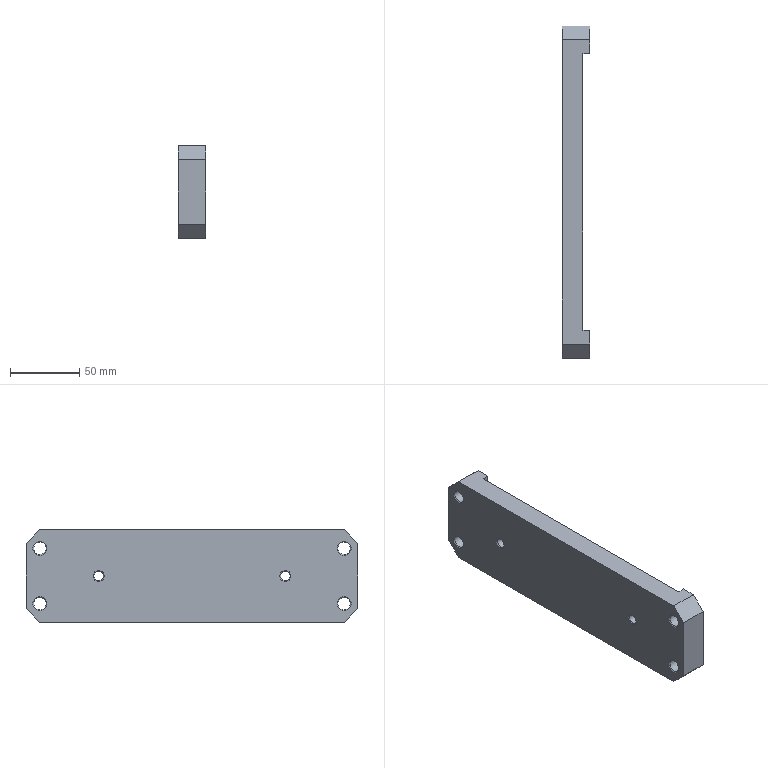Part | NX | features SIMPLE HOLE 6, DATUM_CSYS 5, SKETCH 4, EXTRUDE 2, HOLE PACKAGE 2, LINKED_CURVE 2, SYMBOLIC_THREAD 2, CHAMFER 1, LINKED_FACE 1 | 1 solid | 32 faces | box 20 x 240 x 67 mm | volume 244362 mm3 | plane 14 | cone 12 | cylinder 6 | commonest cylinder face diameters 9 x4 6.8 x2
STEP:
#1=CARTESIAN_POINT('',(85.,-110.,-450.));
#2=VERTEX_POINT('',#1);
#3=CARTESIAN_POINT('',(85.,-100.,-450.));
#4=VERTEX_POINT('',#3);
#5=CARTESIAN_POINT('',(85.,-120.,-450.));
#6=DIRECTION('',(0.,1.,0.));
#7=VECTOR('',#6,1000.);
#8=LINE('',#5,#7);
#9=EDGE_CURVE('',#2,#4,#8,.T.);
#10=ORIENTED_EDGE('',*,*,#9,.F.);
#11=CARTESIAN_POINT('',(65.,-110.,-450.));
#12=VERTEX_POINT('',#11);
#13=CARTESIAN_POINT('',(85.,-110.,-450.));
#14=DIRECTION('',(-1.,0.,0.));
#15=VECTOR('',#14,1000.);
#16=LINE('',#13,#15);
#17=EDGE_CURVE('',#2,#12,#16,.T.);
#18=ORIENTED_EDGE('',*,*,#17,.T.);
#19=CARTESIAN_POINT('',(65.,110.,-450.));
#20=VERTEX_POINT('',#19);
#21=CARTESIAN_POINT('',(65.,-120.,-450.));
#22=DIRECTION('',(0.,1.,0.));
#23=VECTOR('',#22,1000.);
#24=LINE('',#21,#23);
#25=EDGE_CURVE('',#12,#20,#24,.T.);
#26=ORIENTED_EDGE('',*,*,#25,.T.);
#27=CARTESIAN_POINT('',(85.,110.,-450.));
#28=VERTEX_POINT('',#27);
#29=CARTESIAN_POINT('',(85.,110.,-450.));
#30=DIRECTION('',(1.,0.,0.));
#31=VECTOR('',#30,1000.);
#32=LINE('',#29,#31);
#33=EDGE_CURVE('',#20,#28,#32,.T.);
#34=ORIENTED_EDGE('',*,*,#33,.T.);
#35=CARTESIAN_POINT('',(85.,100.,-450.));
#36=VERTEX_POINT('',#35);
#37=CARTESIAN_POINT('',(85.,-120.,-450.));
#38=DIRECTION('',(0.,1.,0.));
#39=VECTOR('',#38,1000.);
#40=LINE('',#37,#39);
#41=EDGE_CURVE('',#36,#28,#40,.T.);
#42=ORIENTED_EDGE('',*,*,#41,.F.);
#43=CARTESIAN_POINT('',(80.,100.,-450.));
#44=VERTEX_POINT('',#43);
#45=CARTESIAN_POINT('',(80.,100.,-450.));
#46=DIRECTION('',(1.,0.,0.));
#47=VECTOR('',#46,1000.);
#48=LINE('',#45,#47);
#49=EDGE_CURVE('',#44,#36,#48,.T.);
#50=ORIENTED_EDGE('',*,*,#49,.F.);
#51=CARTESIAN_POINT('',(80.,-100.,-450.));
#52=VERTEX_POINT('',#51);
#53=CARTESIAN_POINT('',(80.,-100.,-450.));
#54=DIRECTION('',(0.,1.,0.));
#55=VECTOR('',#54,1000.);
#56=LINE('',#53,#55);
#57=EDGE_CURVE('',#52,#44,#56,.T.);
#58=ORIENTED_EDGE('',*,*,#57,.F.);
#59=CARTESIAN_POINT('',(119.,-100.,-450.));
#60=DIRECTION('',(-1.,0.,0.));
#61=VECTOR('',#60,1000.);
#62=LINE('',#59,#61);
#63=EDGE_CURVE('',#4,#52,#62,.T.);
#64=ORIENTED_EDGE('',*,*,#63,.F.);
#65=EDGE_LOOP('',(#10,#18,#26,#34,#42,#50,#58,#64));
#66=FACE_BOUND('',#65,.T.);
#67=CARTESIAN_POINT('',(85.,-120.,-450.));
#68=DIRECTION('',(0.,0.,1.));
#69=DIRECTION('',(0.,-1.,0.));
#70=AXIS2_PLACEMENT_3D('',#67,#68,#69);
#71=PLANE('',#70);
#72=ADVANCED_FACE('',(#66),#71,.F.);
#73=CARTESIAN_POINT('',(85.,110.,-441.6));
#74=VERTEX_POINT('',#73);
#75=CARTESIAN_POINT('',(85.,110.,-436.5));
#76=DIRECTION('',(1.,0.,0.));
#77=DIRECTION('',(0.,0.,-1.));
#78=AXIS2_PLACEMENT_3D('',#75,#76,#77);
#79=CIRCLE('',#78,5.1);
#80=EDGE_CURVE('',#74,#74,#79,.F.);
#81=ORIENTED_EDGE('',*,*,#80,.T.);
#82=EDGE_LOOP('',(#81));
#83=FACE_BOUND('',#82,.T.);
#84=CARTESIAN_POINT('',(85.,110.,-401.6));
#85=VERTEX_POINT('',#84);
#86=CARTESIAN_POINT('',(85.,110.,-396.5));
#87=DIRECTION('',(1.,0.,0.));
#88=DIRECTION('',(0.,0.,-1.));
#89=AXIS2_PLACEMENT_3D('',#86,#87,#88);
#90=CIRCLE('',#89,5.1);
#91=EDGE_CURVE('',#85,#85,#90,.F.);
#92=ORIENTED_EDGE('',*,*,#91,.T.);
#93=EDGE_LOOP('',(#92));
#94=FACE_BOUND('',#93,.T.);
#95=CARTESIAN_POINT('',(85.,120.,-440.));
#96=VERTEX_POINT('',#95);
#97=CARTESIAN_POINT('',(85.,120.,-393.));
#98=VERTEX_POINT('',#97);
#99=CARTESIAN_POINT('',(85.,120.,-450.));
#100=DIRECTION('',(0.,0.,1.));
#101=VECTOR('',#100,1000.);
#102=LINE('',#99,#101);
#103=EDGE_CURVE('',#96,#98,#102,.T.);
#104=ORIENTED_EDGE('',*,*,#103,.T.);
#105=CARTESIAN_POINT('',(85.,110.,-383.));
#106=VERTEX_POINT('',#105);
#107=CARTESIAN_POINT('',(85.,-136.5,-136.5));
#108=DIRECTION('',(0.,0.7071,-0.7071));
#109=VECTOR('',#108,1000.);
#110=LINE('',#107,#109);
#111=EDGE_CURVE('',#98,#106,#110,.F.);
#112=ORIENTED_EDGE('',*,*,#111,.T.);
#113=CARTESIAN_POINT('',(85.,100.,-383.));
#114=VERTEX_POINT('',#113);
#115=CARTESIAN_POINT('',(85.,120.,-383.));
#116=DIRECTION('',(0.,-1.,0.));
#117=VECTOR('',#116,1000.);
#118=LINE('',#115,#117);
#119=EDGE_CURVE('',#106,#114,#118,.T.);
#120=ORIENTED_EDGE('',*,*,#119,.T.);
#121=CARTESIAN_POINT('',(85.,100.,0.));
#122=DIRECTION('',(0.,0.,1.));
#123=VECTOR('',#122,1000.);
#124=LINE('',#121,#123);
#125=EDGE_CURVE('',#36,#114,#124,.T.);
#126=ORIENTED_EDGE('',*,*,#125,.F.);
#127=ORIENTED_EDGE('',*,*,#41,.T.);
#128=CARTESIAN_POINT('',(85.,280.,-280.));
#129=DIRECTION('',(0.,-0.7071,-0.7071));
#130=VECTOR('',#129,1000.);
#131=LINE('',#128,#130);
#132=EDGE_CURVE('',#28,#96,#131,.F.);
#133=ORIENTED_EDGE('',*,*,#132,.T.);
#134=EDGE_LOOP('',(#104,#112,#120,#126,#127,#133));
#135=FACE_BOUND('',#134,.T.);
#136=CARTESIAN_POINT('',(85.,0.,0.));
#137=DIRECTION('',(1.,0.,0.));
#138=DIRECTION('',(0.,0.,-1.));
#139=AXIS2_PLACEMENT_3D('',#136,#137,#138);
#140=PLANE('',#139);
#141=ADVANCED_FACE('',(#83,#94,#135),#140,.T.);
#142=CARTESIAN_POINT('',(85.,-120.,-393.));
#143=VERTEX_POINT('',#142);
#144=CARTESIAN_POINT('',(85.,-120.,-440.));
#145=VERTEX_POINT('',#144);
#146=CARTESIAN_POINT('',(85.,-120.,-383.));
#147=DIRECTION('',(0.,0.,-1.));
#148=VECTOR('',#147,1000.);
#149=LINE('',#146,#148);
#150=EDGE_CURVE('',#143,#145,#149,.T.);
#151=ORIENTED_EDGE('',*,*,#150,.F.);
#152=CARTESIAN_POINT('',(65.,-120.,-393.));
#153=VERTEX_POINT('',#152);
#154=CARTESIAN_POINT('',(85.,-120.,-393.));
#155=DIRECTION('',(-1.,0.,0.));
#156=VECTOR('',#155,1000.);
#157=LINE('',#154,#156);
#158=EDGE_CURVE('',#143,#153,#157,.T.);
#159=ORIENTED_EDGE('',*,*,#158,.T.);
#160=CARTESIAN_POINT('',(65.,-120.,-440.));
#161=VERTEX_POINT('',#160);
#162=CARTESIAN_POINT('',(65.,-120.,-383.));
#163=DIRECTION('',(0.,0.,-1.));
#164=VECTOR('',#163,1000.);
#165=LINE('',#162,#164);
#166=EDGE_CURVE('',#153,#161,#165,.T.);
#167=ORIENTED_EDGE('',*,*,#166,.T.);
#168=CARTESIAN_POINT('',(85.,-120.,-440.));
#169=DIRECTION('',(1.,0.,0.));
#170=VECTOR('',#169,1000.);
#171=LINE('',#168,#170);
#172=EDGE_CURVE('',#161,#145,#171,.T.);
#173=ORIENTED_EDGE('',*,*,#172,.T.);
#174=EDGE_LOOP('',(#151,#159,#167,#173));
#175=FACE_BOUND('',#174,.T.);
#176=CARTESIAN_POINT('',(85.,-120.,-383.));
#177=DIRECTION('',(0.,1.,0.));
#178=DIRECTION('',(0.,0.,1.));
#179=AXIS2_PLACEMENT_3D('',#176,#177,#178);
#180=PLANE('',#179);
#181=ADVANCED_FACE('',(#175),#180,.F.);
#182=CARTESIAN_POINT('',(65.,120.,-440.));
#183=VERTEX_POINT('',#182);
#184=CARTESIAN_POINT('',(65.,120.,-393.));
#185=VERTEX_POINT('',#184);
#186=CARTESIAN_POINT('',(65.,120.,-450.));
#187=DIRECTION('',(0.,0.,1.));
#188=VECTOR('',#187,1000.);
#189=LINE('',#186,#188);
#190=EDGE_CURVE('',#183,#185,#189,.T.);
#191=ORIENTED_EDGE('',*,*,#190,.T.);
#192=CARTESIAN_POINT('',(85.,120.,-393.));
#193=DIRECTION('',(1.,0.,0.));
#194=VECTOR('',#193,1000.);
#195=LINE('',#192,#194);
#196=EDGE_CURVE('',#185,#98,#195,.T.);
#197=ORIENTED_EDGE('',*,*,#196,.T.);
#198=ORIENTED_EDGE('',*,*,#103,.F.);
#199=CARTESIAN_POINT('',(85.,120.,-440.));
#200=DIRECTION('',(-1.,0.,0.));
#201=VECTOR('',#200,1000.);
#202=LINE('',#199,#201);
#203=EDGE_CURVE('',#96,#183,#202,.T.);
#204=ORIENTED_EDGE('',*,*,#203,.T.);
#205=EDGE_LOOP('',(#191,#197,#198,#204));
#206=FACE_BOUND('',#205,.T.);
#207=CARTESIAN_POINT('',(85.,120.,-450.));
#208=DIRECTION('',(0.,-1.,0.));
#209=DIRECTION('',(0.,0.,-1.));
#210=AXIS2_PLACEMENT_3D('',#207,#208,#209);
#211=PLANE('',#210);
#212=ADVANCED_FACE('',(#206),#211,.F.);
#213=CARTESIAN_POINT('',(65.,110.,-383.));
#214=VERTEX_POINT('',#213);
#215=CARTESIAN_POINT('',(65.,-110.,-383.));
#216=VERTEX_POINT('',#215);
#217=CARTESIAN_POINT('',(65.,120.,-383.));
#218=DIRECTION('',(0.,-1.,0.));
#219=VECTOR('',#218,1000.);
#220=LINE('',#217,#219);
#221=EDGE_CURVE('',#214,#216,#220,.T.);
#222=ORIENTED_EDGE('',*,*,#221,.T.);
#223=CARTESIAN_POINT('',(85.,-110.,-383.));
#224=VERTEX_POINT('',#223);
#225=CARTESIAN_POINT('',(85.,-110.,-383.));
#226=DIRECTION('',(1.,0.,0.));
#227=VECTOR('',#226,1000.);
#228=LINE('',#225,#227);
#229=EDGE_CURVE('',#216,#224,#228,.T.);
#230=ORIENTED_EDGE('',*,*,#229,.T.);
#231=CARTESIAN_POINT('',(85.,-100.,-383.));
#232=VERTEX_POINT('',#231);
#233=CARTESIAN_POINT('',(85.,120.,-383.));
#234=DIRECTION('',(0.,-1.,0.));
#235=VECTOR('',#234,1000.);
#236=LINE('',#233,#235);
#237=EDGE_CURVE('',#232,#224,#236,.T.);
#238=ORIENTED_EDGE('',*,*,#237,.F.);
#239=CARTESIAN_POINT('',(80.,-100.,-383.));
#240=VERTEX_POINT('',#239);
#241=CARTESIAN_POINT('',(85.,-100.,-383.));
#242=DIRECTION('',(-1.,0.,0.));
#243=VECTOR('',#242,1000.);
#244=LINE('',#241,#243);
#245=EDGE_CURVE('',#232,#240,#244,.T.);
#246=ORIENTED_EDGE('',*,*,#245,.T.);
#247=CARTESIAN_POINT('',(80.,100.,-383.));
#248=VERTEX_POINT('',#247);
#249=CARTESIAN_POINT('',(80.,120.,-383.));
#250=DIRECTION('',(0.,1.,0.));
#251=VECTOR('',#250,1000.);
#252=LINE('',#249,#251);
#253=EDGE_CURVE('',#240,#248,#252,.T.);
#254=ORIENTED_EDGE('',*,*,#253,.T.);
#255=CARTESIAN_POINT('',(85.,100.,-383.));
#256=DIRECTION('',(1.,0.,0.));
#257=VECTOR('',#256,1000.);
#258=LINE('',#255,#257);
#259=EDGE_CURVE('',#248,#114,#258,.T.);
#260=ORIENTED_EDGE('',*,*,#259,.T.);
#261=ORIENTED_EDGE('',*,*,#119,.F.);
#262=CARTESIAN_POINT('',(85.,110.,-383.));
#263=DIRECTION('',(-1.,0.,0.));
#264=VECTOR('',#263,1000.);
#265=LINE('',#262,#264);
#266=EDGE_CURVE('',#106,#214,#265,.T.);
#267=ORIENTED_EDGE('',*,*,#266,.T.);
#268=EDGE_LOOP('',(#222,#230,#238,#246,#254,#260,#261,#267));
#269=FACE_BOUND('',#268,.T.);
#270=CARTESIAN_POINT('',(85.,120.,-383.));
#271=DIRECTION('',(0.,0.,-1.));
#272=DIRECTION('',(-1.,0.,0.));
#273=AXIS2_PLACEMENT_3D('',#270,#271,#272);
#274=PLANE('',#273);
#275=ADVANCED_FACE('',(#269),#274,.F.);
#276=CARTESIAN_POINT('',(85.,-110.,-441.6));
#277=VERTEX_POINT('',#276);
#278=CARTESIAN_POINT('',(85.,-110.,-436.5));
#279=DIRECTION('',(1.,0.,0.));
#280=DIRECTION('',(0.,0.,-1.));
#281=AXIS2_PLACEMENT_3D('',#278,#279,#280);
#282=CIRCLE('',#281,5.1);
#283=EDGE_CURVE('',#277,#277,#282,.F.);
#284=ORIENTED_EDGE('',*,*,#283,.T.);
#285=EDGE_LOOP('',(#284));
#286=FACE_BOUND('',#285,.T.);
#287=CARTESIAN_POINT('',(85.,-110.,-401.6));
#288=VERTEX_POINT('',#287);
#289=CARTESIAN_POINT('',(85.,-110.,-396.5));
#290=DIRECTION('',(1.,0.,0.));
#291=DIRECTION('',(0.,0.,-1.));
#292=AXIS2_PLACEMENT_3D('',#289,#290,#291);
#293=CIRCLE('',#292,5.1);
#294=EDGE_CURVE('',#288,#288,#293,.F.);
#295=ORIENTED_EDGE('',*,*,#294,.T.);
#296=EDGE_LOOP('',(#295));
#297=FACE_BOUND('',#296,.T.);
#298=ORIENTED_EDGE('',*,*,#237,.T.);
#299=CARTESIAN_POINT('',(85.,136.5,-136.5));
#300=DIRECTION('',(0.,0.7071,0.7071));
#301=VECTOR('',#300,1000.);
#302=LINE('',#299,#301);
#303=EDGE_CURVE('',#224,#143,#302,.F.);
#304=ORIENTED_EDGE('',*,*,#303,.T.);
#305=ORIENTED_EDGE('',*,*,#150,.T.);
#306=CARTESIAN_POINT('',(85.,-280.,-280.));
#307=DIRECTION('',(0.,-0.7071,0.7071));
#308=VECTOR('',#307,1000.);
#309=LINE('',#306,#308);
#310=EDGE_CURVE('',#145,#2,#309,.F.);
#311=ORIENTED_EDGE('',*,*,#310,.T.);
#312=ORIENTED_EDGE('',*,*,#9,.T.);
#313=CARTESIAN_POINT('',(85.,-100.,0.));
#314=DIRECTION('',(0.,0.,-1.));
#315=VECTOR('',#314,1000.);
#316=LINE('',#313,#315);
#317=EDGE_CURVE('',#232,#4,#316,.T.);
#318=ORIENTED_EDGE('',*,*,#317,.F.);
#319=EDGE_LOOP('',(#298,#304,#305,#311,#312,#318));
#320=FACE_BOUND('',#319,.T.);
#321=CARTESIAN_POINT('',(85.,0.,0.));
#322=DIRECTION('',(1.,0.,0.));
#323=DIRECTION('',(0.,0.,-1.));
#324=AXIS2_PLACEMENT_3D('',#321,#322,#323);
#325=PLANE('',#324);
#326=ADVANCED_FACE('',(#286,#297,#320),#325,.T.);
#327=CARTESIAN_POINT('',(65.,-110.,-441.6));
#328=VERTEX_POINT('',#327);
#329=CARTESIAN_POINT('',(65.,-110.,-436.5));
#330=DIRECTION('',(1.,0.,0.));
#331=DIRECTION('',(0.,0.,-1.));
#332=AXIS2_PLACEMENT_3D('',#329,#330,#331);
#333=CIRCLE('',#332,5.1);
#334=EDGE_CURVE('',#328,#328,#333,.T.);
#335=ORIENTED_EDGE('',*,*,#334,.T.);
#336=EDGE_LOOP('',(#335));
#337=FACE_BOUND('',#336,.T.);
#338=CARTESIAN_POINT('',(65.,-110.,-401.6));
#339=VERTEX_POINT('',#338);
#340=CARTESIAN_POINT('',(65.,-110.,-396.5));
#341=DIRECTION('',(1.,0.,0.));
#342=DIRECTION('',(0.,0.,-1.));
#343=AXIS2_PLACEMENT_3D('',#340,#341,#342);
#344=CIRCLE('',#343,5.1);
#345=EDGE_CURVE('',#339,#339,#344,.T.);
#346=ORIENTED_EDGE('',*,*,#345,.T.);
#347=EDGE_LOOP('',(#346));
#348=FACE_BOUND('',#347,.T.);
#349=CARTESIAN_POINT('',(65.,110.,-441.6));
#350=VERTEX_POINT('',#349);
#351=CARTESIAN_POINT('',(65.,110.,-436.5));
#352=DIRECTION('',(1.,0.,0.));
#353=DIRECTION('',(0.,0.,-1.));
#354=AXIS2_PLACEMENT_3D('',#351,#352,#353);
#355=CIRCLE('',#354,5.1);
#356=EDGE_CURVE('',#350,#350,#355,.T.);
#357=ORIENTED_EDGE('',*,*,#356,.T.);
#358=EDGE_LOOP('',(#357));
#359=FACE_BOUND('',#358,.T.);
#360=CARTESIAN_POINT('',(65.,110.,-401.6));
#361=VERTEX_POINT('',#360);
#362=CARTESIAN_POINT('',(65.,110.,-396.5));
#363=DIRECTION('',(1.,0.,0.));
#364=DIRECTION('',(0.,0.,-1.));
#365=AXIS2_PLACEMENT_3D('',#362,#363,#364);
#366=CIRCLE('',#365,5.1);
#367=EDGE_CURVE('',#361,#361,#366,.T.);
#368=ORIENTED_EDGE('',*,*,#367,.T.);
#369=EDGE_LOOP('',(#368));
#370=FACE_BOUND('',#369,.T.);
#371=CARTESIAN_POINT('',(65.,67.5,-420.5));
#372=VERTEX_POINT('',#371);
#373=CARTESIAN_POINT('',(65.,67.5,-416.5));
#374=DIRECTION('',(1.,0.,0.));
#375=DIRECTION('',(0.,0.,-1.));
#376=AXIS2_PLACEMENT_3D('',#373,#374,#375);
#377=CIRCLE('',#376,4.);
#378=EDGE_CURVE('',#372,#372,#377,.T.);
#379=ORIENTED_EDGE('',*,*,#378,.T.);
#380=EDGE_LOOP('',(#379));
#381=FACE_BOUND('',#380,.T.);
#382=CARTESIAN_POINT('',(65.,-67.5,-420.5));
#383=VERTEX_POINT('',#382);
#384=CARTESIAN_POINT('',(65.,-67.5,-416.5));
#385=DIRECTION('',(1.,0.,0.));
#386=DIRECTION('',(0.,0.,-1.));
#387=AXIS2_PLACEMENT_3D('',#384,#385,#386);
#388=CIRCLE('',#387,4.);
#389=EDGE_CURVE('',#383,#383,#388,.T.);
#390=ORIENTED_EDGE('',*,*,#389,.T.);
#391=EDGE_LOOP('',(#390));
#392=FACE_BOUND('',#391,.T.);
#393=ORIENTED_EDGE('',*,*,#166,.F.);
#394=CARTESIAN_POINT('',(65.,-120.,-393.));
#395=DIRECTION('',(0.,-0.7071,-0.7071));
#396=VECTOR('',#395,1000.);
#397=LINE('',#394,#396);
#398=EDGE_CURVE('',#153,#216,#397,.F.);
#399=ORIENTED_EDGE('',*,*,#398,.T.);
#400=ORIENTED_EDGE('',*,*,#221,.F.);
#401=CARTESIAN_POINT('',(65.,110.,-383.));
#402=DIRECTION('',(0.,-0.7071,0.7071));
#403=VECTOR('',#402,1000.);
#404=LINE('',#401,#403);
#405=EDGE_CURVE('',#214,#185,#404,.F.);
#406=ORIENTED_EDGE('',*,*,#405,.T.);
#407=ORIENTED_EDGE('',*,*,#190,.F.);
#408=CARTESIAN_POINT('',(65.,120.,-440.));
#409=DIRECTION('',(0.,0.7071,0.7071));
#410=VECTOR('',#409,1000.);
#411=LINE('',#408,#410);
#412=EDGE_CURVE('',#183,#20,#411,.F.);
#413=ORIENTED_EDGE('',*,*,#412,.T.);
#414=ORIENTED_EDGE('',*,*,#25,.F.);
#415=CARTESIAN_POINT('',(65.,-110.,-450.));
#416=DIRECTION('',(0.,0.7071,-0.7071));
#417=VECTOR('',#416,1000.);
#418=LINE('',#415,#417);
#419=EDGE_CURVE('',#12,#161,#418,.F.);
#420=ORIENTED_EDGE('',*,*,#419,.T.);
#421=EDGE_LOOP('',(#393,#399,#400,#406,#407,#413,#414,#420));
#422=FACE_BOUND('',#421,.T.);
#423=CARTESIAN_POINT('',(65.,0.,0.));
#424=DIRECTION('',(1.,0.,0.));
#425=DIRECTION('',(0.,0.,-1.));
#426=AXIS2_PLACEMENT_3D('',#423,#424,#425);
#427=PLANE('',#426);
#428=ADVANCED_FACE('',(#337,#348,#359,#370,#381,#392,#422),#427,.F.);
#429=CARTESIAN_POINT('',(80.,63.5,-416.5));
#430=VERTEX_POINT('',#429);
#431=CARTESIAN_POINT('',(80.,67.5,-416.5));
#432=DIRECTION('',(-1.,0.,0.));
#433=DIRECTION('',(0.,-1.,0.));
#434=AXIS2_PLACEMENT_3D('',#431,#432,#433);
#435=CIRCLE('',#434,4.);
#436=EDGE_CURVE('',#430,#430,#435,.T.);
#437=ORIENTED_EDGE('',*,*,#436,.T.);
#438=EDGE_LOOP('',(#437));
#439=FACE_BOUND('',#438,.T.);
#440=CARTESIAN_POINT('',(80.,-71.5,-416.5));
#441=VERTEX_POINT('',#440);
#442=CARTESIAN_POINT('',(80.,-67.5,-416.5));
#443=DIRECTION('',(-1.,0.,0.));
#444=DIRECTION('',(0.,-1.,0.));
#445=AXIS2_PLACEMENT_3D('',#442,#443,#444);
#446=CIRCLE('',#445,4.);
#447=EDGE_CURVE('',#441,#441,#446,.T.);
#448=ORIENTED_EDGE('',*,*,#447,.T.);
#449=EDGE_LOOP('',(#448));
#450=FACE_BOUND('',#449,.T.);
#451=CARTESIAN_POINT('',(80.,-100.,-255.));
#452=DIRECTION('',(0.,0.,-1.));
#453=VECTOR('',#452,1000.);
#454=LINE('',#451,#453);
#455=EDGE_CURVE('',#52,#240,#454,.F.);
#456=ORIENTED_EDGE('',*,*,#455,.F.);
#457=ORIENTED_EDGE('',*,*,#57,.T.);
#458=CARTESIAN_POINT('',(80.,100.,-255.));
#459=DIRECTION('',(0.,0.,-1.));
#460=VECTOR('',#459,1000.);
#461=LINE('',#458,#460);
#462=EDGE_CURVE('',#44,#248,#461,.F.);
#463=ORIENTED_EDGE('',*,*,#462,.T.);
#464=ORIENTED_EDGE('',*,*,#253,.F.);
#465=EDGE_LOOP('',(#456,#457,#463,#464));
#466=FACE_BOUND('',#465,.T.);
#467=CARTESIAN_POINT('',(80.,-100.,-255.));
#468=DIRECTION('',(-1.,0.,0.));
#469=DIRECTION('',(0.,-1.,0.));
#470=AXIS2_PLACEMENT_3D('',#467,#468,#469);
#471=PLANE('',#470);
#472=ADVANCED_FACE('',(#439,#450,#466),#471,.F.);
#473=ORIENTED_EDGE('',*,*,#462,.F.);
#474=ORIENTED_EDGE('',*,*,#49,.T.);
#475=ORIENTED_EDGE('',*,*,#125,.T.);
#476=ORIENTED_EDGE('',*,*,#259,.F.);
#477=EDGE_LOOP('',(#473,#474,#475,#476));
#478=FACE_BOUND('',#477,.T.);
#479=CARTESIAN_POINT('',(80.,100.,-255.));
#480=DIRECTION('',(0.,1.,0.));
#481=DIRECTION('',(0.,0.,1.));
#482=AXIS2_PLACEMENT_3D('',#479,#480,#481);
#483=PLANE('',#482);
#484=ADVANCED_FACE('',(#478),#483,.F.);
#485=ORIENTED_EDGE('',*,*,#317,.T.);
#486=ORIENTED_EDGE('',*,*,#63,.T.);
#487=ORIENTED_EDGE('',*,*,#455,.T.);
#488=ORIENTED_EDGE('',*,*,#245,.F.);
#489=EDGE_LOOP('',(#485,#486,#487,#488));
#490=FACE_BOUND('',#489,.T.);
#491=CARTESIAN_POINT('',(119.,-100.,-255.));
#492=DIRECTION('',(0.,-1.,0.));
#493=DIRECTION('',(0.,0.,-1.));
#494=AXIS2_PLACEMENT_3D('',#491,#492,#493);
#495=PLANE('',#494);
#496=ADVANCED_FACE('',(#490),#495,.F.);
#497=ORIENTED_EDGE('',*,*,#303,.F.);
#498=ORIENTED_EDGE('',*,*,#229,.F.);
#499=ORIENTED_EDGE('',*,*,#398,.F.);
#500=ORIENTED_EDGE('',*,*,#158,.F.);
#501=EDGE_LOOP('',(#497,#498,#499,#500));
#502=FACE_BOUND('',#501,.T.);
#503=CARTESIAN_POINT('',(85.,-120.,-393.));
#504=DIRECTION('',(0.,0.7071,-0.7071));
#505=DIRECTION('',(-1.,0.,0.));
#506=AXIS2_PLACEMENT_3D('',#503,#504,#505);
#507=PLANE('',#506);
#508=ADVANCED_FACE('',(#502),#507,.F.);
#509=ORIENTED_EDGE('',*,*,#310,.F.);
#510=ORIENTED_EDGE('',*,*,#172,.F.);
#511=ORIENTED_EDGE('',*,*,#419,.F.);
#512=ORIENTED_EDGE('',*,*,#17,.F.);
#513=EDGE_LOOP('',(#509,#510,#511,#512));
#514=FACE_BOUND('',#513,.T.);
#515=CARTESIAN_POINT('',(85.,-110.,-450.));
#516=DIRECTION('',(0.,0.7071,0.7071));
#517=DIRECTION('',(-1.,0.,0.));
#518=AXIS2_PLACEMENT_3D('',#515,#516,#517);
#519=PLANE('',#518);
#520=ADVANCED_FACE('',(#514),#519,.F.);
#521=ORIENTED_EDGE('',*,*,#111,.F.);
#522=ORIENTED_EDGE('',*,*,#196,.F.);
#523=ORIENTED_EDGE('',*,*,#405,.F.);
#524=ORIENTED_EDGE('',*,*,#266,.F.);
#525=EDGE_LOOP('',(#521,#522,#523,#524));
#526=FACE_BOUND('',#525,.T.);
#527=CARTESIAN_POINT('',(85.,110.,-383.));
#528=DIRECTION('',(0.,-0.7071,-0.7071));
#529=DIRECTION('',(-1.,0.,0.));
#530=AXIS2_PLACEMENT_3D('',#527,#528,#529);
#531=PLANE('',#530);
#532=ADVANCED_FACE('',(#526),#531,.F.);
#533=ORIENTED_EDGE('',*,*,#132,.F.);
#534=ORIENTED_EDGE('',*,*,#33,.F.);
#535=ORIENTED_EDGE('',*,*,#412,.F.);
#536=ORIENTED_EDGE('',*,*,#203,.F.);
#537=EDGE_LOOP('',(#533,#534,#535,#536));
#538=FACE_BOUND('',#537,.T.);
#539=CARTESIAN_POINT('',(85.,120.,-440.));
#540=DIRECTION('',(0.,-0.7071,0.7071));
#541=DIRECTION('',(-1.,0.,0.));
#542=AXIS2_PLACEMENT_3D('',#539,#540,#541);
#543=PLANE('',#542);
#544=ADVANCED_FACE('',(#538),#543,.F.);
#545=CARTESIAN_POINT('',(79.4,-67.5,-413.1));
#546=VERTEX_POINT('',#545);
#547=CARTESIAN_POINT('',(79.4,-67.5,-416.5));
#548=DIRECTION('',(-1.,0.,0.));
#549=DIRECTION('',(0.,0.,1.));
#550=AXIS2_PLACEMENT_3D('',#547,#548,#549);
#551=CIRCLE('',#550,3.4);
#552=EDGE_CURVE('',#546,#546,#551,.F.);
#553=ORIENTED_EDGE('',*,*,#552,.T.);
#554=EDGE_LOOP('',(#553));
#555=FACE_BOUND('',#554,.T.);
#556=CARTESIAN_POINT('',(65.6,-67.5,-419.9));
#557=VERTEX_POINT('',#556);
#558=CARTESIAN_POINT('',(65.6,-67.5,-416.5));
#559=DIRECTION('',(1.,0.,0.));
#560=DIRECTION('',(0.,0.,-1.));
#561=AXIS2_PLACEMENT_3D('',#558,#559,#560);
#562=CIRCLE('',#561,3.4);
#563=EDGE_CURVE('',#557,#557,#562,.F.);
#564=ORIENTED_EDGE('',*,*,#563,.T.);
#565=EDGE_LOOP('',(#564));
#566=FACE_BOUND('',#565,.T.);
#567=CARTESIAN_POINT('',(65.,-67.5,-416.5));
#568=DIRECTION('',(1.,0.,0.));
#569=DIRECTION('',(0.,0.,-1.));
#570=AXIS2_PLACEMENT_3D('',#567,#568,#569);
#571=CYLINDRICAL_SURFACE('',#570,3.4);
#572=ADVANCED_FACE('',(#555,#566),#571,.F.);
#573=ORIENTED_EDGE('',*,*,#563,.F.);
#574=EDGE_LOOP('',(#573));
#575=FACE_BOUND('',#574,.T.);
#576=ORIENTED_EDGE('',*,*,#389,.F.);
#577=EDGE_LOOP('',(#576));
#578=FACE_BOUND('',#577,.T.);
#579=CARTESIAN_POINT('',(65.,-67.5,-416.5));
#580=DIRECTION('',(-1.,0.,0.));
#581=DIRECTION('',(0.,0.,1.));
#582=AXIS2_PLACEMENT_3D('',#579,#580,#581);
#583=CONICAL_SURFACE('',#582,4.,0.7854);
#584=ADVANCED_FACE('',(#575,#578),#583,.F.);
#585=ORIENTED_EDGE('',*,*,#552,.F.);
#586=EDGE_LOOP('',(#585));
#587=FACE_BOUND('',#586,.T.);
#588=ORIENTED_EDGE('',*,*,#447,.F.);
#589=EDGE_LOOP('',(#588));
#590=FACE_BOUND('',#589,.T.);
#591=CARTESIAN_POINT('',(80.,-67.5,-416.5));
#592=DIRECTION('',(1.,0.,0.));
#593=DIRECTION('',(0.,0.,-1.));
#594=AXIS2_PLACEMENT_3D('',#591,#592,#593);
#595=CONICAL_SURFACE('',#594,4.,0.7854);
#596=ADVANCED_FACE('',(#587,#590),#595,.F.);
#597=CARTESIAN_POINT('',(79.4,67.5,-413.1));
#598=VERTEX_POINT('',#597);
#599=CARTESIAN_POINT('',(79.4,67.5,-416.5));
#600=DIRECTION('',(-1.,0.,0.));
#601=DIRECTION('',(0.,0.,1.));
#602=AXIS2_PLACEMENT_3D('',#599,#600,#601);
#603=CIRCLE('',#602,3.4);
#604=EDGE_CURVE('',#598,#598,#603,.F.);
#605=ORIENTED_EDGE('',*,*,#604,.T.);
#606=EDGE_LOOP('',(#605));
#607=FACE_BOUND('',#606,.T.);
#608=CARTESIAN_POINT('',(65.6,67.5,-419.9));
#609=VERTEX_POINT('',#608);
#610=CARTESIAN_POINT('',(65.6,67.5,-416.5));
#611=DIRECTION('',(1.,0.,0.));
#612=DIRECTION('',(0.,0.,-1.));
#613=AXIS2_PLACEMENT_3D('',#610,#611,#612);
#614=CIRCLE('',#613,3.4);
#615=EDGE_CURVE('',#609,#609,#614,.F.);
#616=ORIENTED_EDGE('',*,*,#615,.T.);
#617=EDGE_LOOP('',(#616));
#618=FACE_BOUND('',#617,.T.);
#619=CARTESIAN_POINT('',(65.,67.5,-416.5));
#620=DIRECTION('',(1.,0.,0.));
#621=DIRECTION('',(0.,0.,-1.));
#622=AXIS2_PLACEMENT_3D('',#619,#620,#621);
#623=CYLINDRICAL_SURFACE('',#622,3.4);
#624=ADVANCED_FACE('',(#607,#618),#623,.F.);
#625=ORIENTED_EDGE('',*,*,#615,.F.);
#626=EDGE_LOOP('',(#625));
#627=FACE_BOUND('',#626,.T.);
#628=ORIENTED_EDGE('',*,*,#378,.F.);
#629=EDGE_LOOP('',(#628));
#630=FACE_BOUND('',#629,.T.);
#631=CARTESIAN_POINT('',(65.,67.5,-416.5));
#632=DIRECTION('',(-1.,0.,0.));
#633=DIRECTION('',(0.,0.,1.));
#634=AXIS2_PLACEMENT_3D('',#631,#632,#633);
#635=CONICAL_SURFACE('',#634,4.,0.7854);
#636=ADVANCED_FACE('',(#627,#630),#635,.F.);
#637=ORIENTED_EDGE('',*,*,#604,.F.);
#638=EDGE_LOOP('',(#637));
#639=FACE_BOUND('',#638,.T.);
#640=ORIENTED_EDGE('',*,*,#436,.F.);
#641=EDGE_LOOP('',(#640));
#642=FACE_BOUND('',#641,.T.);
#643=CARTESIAN_POINT('',(80.,67.5,-416.5));
#644=DIRECTION('',(1.,0.,0.));
#645=DIRECTION('',(0.,0.,-1.));
#646=AXIS2_PLACEMENT_3D('',#643,#644,#645);
#647=CONICAL_SURFACE('',#646,4.,0.7854);
#648=ADVANCED_FACE('',(#639,#642),#647,.F.);
#649=CARTESIAN_POINT('',(84.4,110.,-401.));
#650=VERTEX_POINT('',#649);
#651=CARTESIAN_POINT('',(84.4,110.,-396.5));
#652=DIRECTION('',(1.,0.,0.));
#653=DIRECTION('',(0.,0.,-1.));
#654=AXIS2_PLACEMENT_3D('',#651,#652,#653);
#655=CIRCLE('',#654,4.5);
#656=EDGE_CURVE('',#650,#650,#655,.T.);
#657=ORIENTED_EDGE('',*,*,#656,.T.);
#658=EDGE_LOOP('',(#657));
#659=FACE_BOUND('',#658,.T.);
#660=CARTESIAN_POINT('',(65.6,110.,-401.));
#661=VERTEX_POINT('',#660);
#662=CARTESIAN_POINT('',(65.6,110.,-396.5));
#663=DIRECTION('',(1.,0.,0.));
#664=DIRECTION('',(0.,0.,-1.));
#665=AXIS2_PLACEMENT_3D('',#662,#663,#664);
#666=CIRCLE('',#665,4.5);
#667=EDGE_CURVE('',#661,#661,#666,.F.);
#668=ORIENTED_EDGE('',*,*,#667,.T.);
#669=EDGE_LOOP('',(#668));
#670=FACE_BOUND('',#669,.T.);
#671=CARTESIAN_POINT('',(65.,110.,-396.5));
#672=DIRECTION('',(1.,0.,0.));
#673=DIRECTION('',(0.,0.,-1.));
#674=AXIS2_PLACEMENT_3D('',#671,#672,#673);
#675=CYLINDRICAL_SURFACE('',#674,4.5);
#676=ADVANCED_FACE('',(#659,#670),#675,.F.);
#677=ORIENTED_EDGE('',*,*,#667,.F.);
#678=EDGE_LOOP('',(#677));
#679=FACE_BOUND('',#678,.T.);
#680=ORIENTED_EDGE('',*,*,#367,.F.);
#681=EDGE_LOOP('',(#680));
#682=FACE_BOUND('',#681,.T.);
#683=CARTESIAN_POINT('',(65.,110.,-396.5));
#684=DIRECTION('',(-1.,0.,0.));
#685=DIRECTION('',(0.,0.,1.));
#686=AXIS2_PLACEMENT_3D('',#683,#684,#685);
#687=CONICAL_SURFACE('',#686,5.1,0.7854);
#688=ADVANCED_FACE('',(#679,#682),#687,.F.);
#689=ORIENTED_EDGE('',*,*,#91,.F.);
#690=EDGE_LOOP('',(#689));
#691=FACE_BOUND('',#690,.T.);
#692=ORIENTED_EDGE('',*,*,#656,.F.);
#693=EDGE_LOOP('',(#692));
#694=FACE_BOUND('',#693,.T.);
#695=CARTESIAN_POINT('',(84.4,110.,-396.5));
#696=DIRECTION('',(1.,0.,0.));
#697=DIRECTION('',(0.,0.,-1.));
#698=AXIS2_PLACEMENT_3D('',#695,#696,#697);
#699=CONICAL_SURFACE('',#698,4.5,0.7854);
#700=ADVANCED_FACE('',(#691,#694),#699,.F.);
#701=CARTESIAN_POINT('',(84.4,110.,-441.));
#702=VERTEX_POINT('',#701);
#703=CARTESIAN_POINT('',(84.4,110.,-436.5));
#704=DIRECTION('',(1.,0.,0.));
#705=DIRECTION('',(0.,0.,-1.));
#706=AXIS2_PLACEMENT_3D('',#703,#704,#705);
#707=CIRCLE('',#706,4.5);
#708=EDGE_CURVE('',#702,#702,#707,.T.);
#709=ORIENTED_EDGE('',*,*,#708,.T.);
#710=EDGE_LOOP('',(#709));
#711=FACE_BOUND('',#710,.T.);
#712=CARTESIAN_POINT('',(65.6,110.,-441.));
#713=VERTEX_POINT('',#712);
#714=CARTESIAN_POINT('',(65.6,110.,-436.5));
#715=DIRECTION('',(1.,0.,0.));
#716=DIRECTION('',(0.,0.,-1.));
#717=AXIS2_PLACEMENT_3D('',#714,#715,#716);
#718=CIRCLE('',#717,4.5);
#719=EDGE_CURVE('',#713,#713,#718,.F.);
#720=ORIENTED_EDGE('',*,*,#719,.T.);
#721=EDGE_LOOP('',(#720));
#722=FACE_BOUND('',#721,.T.);
#723=CARTESIAN_POINT('',(65.,110.,-436.5));
#724=DIRECTION('',(1.,0.,0.));
#725=DIRECTION('',(0.,0.,-1.));
#726=AXIS2_PLACEMENT_3D('',#723,#724,#725);
#727=CYLINDRICAL_SURFACE('',#726,4.5);
#728=ADVANCED_FACE('',(#711,#722),#727,.F.);
#729=ORIENTED_EDGE('',*,*,#719,.F.);
#730=EDGE_LOOP('',(#729));
#731=FACE_BOUND('',#730,.T.);
#732=ORIENTED_EDGE('',*,*,#356,.F.);
#733=EDGE_LOOP('',(#732));
#734=FACE_BOUND('',#733,.T.);
#735=CARTESIAN_POINT('',(65.,110.,-436.5));
#736=DIRECTION('',(-1.,0.,0.));
#737=DIRECTION('',(0.,0.,1.));
#738=AXIS2_PLACEMENT_3D('',#735,#736,#737);
#739=CONICAL_SURFACE('',#738,5.1,0.7854);
#740=ADVANCED_FACE('',(#731,#734),#739,.F.);
#741=ORIENTED_EDGE('',*,*,#80,.F.);
#742=EDGE_LOOP('',(#741));
#743=FACE_BOUND('',#742,.T.);
#744=ORIENTED_EDGE('',*,*,#708,.F.);
#745=EDGE_LOOP('',(#744));
#746=FACE_BOUND('',#745,.T.);
#747=CARTESIAN_POINT('',(84.4,110.,-436.5));
#748=DIRECTION('',(1.,0.,0.));
#749=DIRECTION('',(0.,0.,-1.));
#750=AXIS2_PLACEMENT_3D('',#747,#748,#749);
#751=CONICAL_SURFACE('',#750,4.5,0.7854);
#752=ADVANCED_FACE('',(#743,#746),#751,.F.);
#753=CARTESIAN_POINT('',(84.4,-110.,-401.));
#754=VERTEX_POINT('',#753);
#755=CARTESIAN_POINT('',(84.4,-110.,-396.5));
#756=DIRECTION('',(1.,0.,0.));
#757=DIRECTION('',(0.,0.,-1.));
#758=AXIS2_PLACEMENT_3D('',#755,#756,#757);
#759=CIRCLE('',#758,4.5);
#760=EDGE_CURVE('',#754,#754,#759,.T.);
#761=ORIENTED_EDGE('',*,*,#760,.T.);
#762=EDGE_LOOP('',(#761));
#763=FACE_BOUND('',#762,.T.);
#764=CARTESIAN_POINT('',(65.6,-110.,-401.));
#765=VERTEX_POINT('',#764);
#766=CARTESIAN_POINT('',(65.6,-110.,-396.5));
#767=DIRECTION('',(1.,0.,0.));
#768=DIRECTION('',(0.,0.,-1.));
#769=AXIS2_PLACEMENT_3D('',#766,#767,#768);
#770=CIRCLE('',#769,4.5);
#771=EDGE_CURVE('',#765,#765,#770,.F.);
#772=ORIENTED_EDGE('',*,*,#771,.T.);
#773=EDGE_LOOP('',(#772));
#774=FACE_BOUND('',#773,.T.);
#775=CARTESIAN_POINT('',(65.,-110.,-396.5));
#776=DIRECTION('',(1.,0.,0.));
#777=DIRECTION('',(0.,0.,-1.));
#778=AXIS2_PLACEMENT_3D('',#775,#776,#777);
#779=CYLINDRICAL_SURFACE('',#778,4.5);
#780=ADVANCED_FACE('',(#763,#774),#779,.F.);
#781=ORIENTED_EDGE('',*,*,#771,.F.);
#782=EDGE_LOOP('',(#781));
#783=FACE_BOUND('',#782,.T.);
#784=ORIENTED_EDGE('',*,*,#345,.F.);
#785=EDGE_LOOP('',(#784));
#786=FACE_BOUND('',#785,.T.);
#787=CARTESIAN_POINT('',(65.,-110.,-396.5));
#788=DIRECTION('',(-1.,0.,0.));
#789=DIRECTION('',(0.,0.,1.));
#790=AXIS2_PLACEMENT_3D('',#787,#788,#789);
#791=CONICAL_SURFACE('',#790,5.1,0.7854);
#792=ADVANCED_FACE('',(#783,#786),#791,.F.);
#793=ORIENTED_EDGE('',*,*,#294,.F.);
#794=EDGE_LOOP('',(#793));
#795=FACE_BOUND('',#794,.T.);
#796=ORIENTED_EDGE('',*,*,#760,.F.);
#797=EDGE_LOOP('',(#796));
#798=FACE_BOUND('',#797,.T.);
#799=CARTESIAN_POINT('',(84.4,-110.,-396.5));
#800=DIRECTION('',(1.,0.,0.));
#801=DIRECTION('',(0.,0.,-1.));
#802=AXIS2_PLACEMENT_3D('',#799,#800,#801);
#803=CONICAL_SURFACE('',#802,4.5,0.7854);
#804=ADVANCED_FACE('',(#795,#798),#803,.F.);
#805=CARTESIAN_POINT('',(84.4,-110.,-441.));
#806=VERTEX_POINT('',#805);
#807=CARTESIAN_POINT('',(84.4,-110.,-436.5));
#808=DIRECTION('',(1.,0.,0.));
#809=DIRECTION('',(0.,0.,-1.));
#810=AXIS2_PLACEMENT_3D('',#807,#808,#809);
#811=CIRCLE('',#810,4.5);
#812=EDGE_CURVE('',#806,#806,#811,.T.);
#813=ORIENTED_EDGE('',*,*,#812,.T.);
#814=EDGE_LOOP('',(#813));
#815=FACE_BOUND('',#814,.T.);
#816=CARTESIAN_POINT('',(65.6,-110.,-441.));
#817=VERTEX_POINT('',#816);
#818=CARTESIAN_POINT('',(65.6,-110.,-436.5));
#819=DIRECTION('',(1.,0.,0.));
#820=DIRECTION('',(0.,0.,-1.));
#821=AXIS2_PLACEMENT_3D('',#818,#819,#820);
#822=CIRCLE('',#821,4.5);
#823=EDGE_CURVE('',#817,#817,#822,.F.);
#824=ORIENTED_EDGE('',*,*,#823,.T.);
#825=EDGE_LOOP('',(#824));
#826=FACE_BOUND('',#825,.T.);
#827=CARTESIAN_POINT('',(65.,-110.,-436.5));
#828=DIRECTION('',(1.,0.,0.));
#829=DIRECTION('',(0.,0.,-1.));
#830=AXIS2_PLACEMENT_3D('',#827,#828,#829);
#831=CYLINDRICAL_SURFACE('',#830,4.5);
#832=ADVANCED_FACE('',(#815,#826),#831,.F.);
#833=ORIENTED_EDGE('',*,*,#823,.F.);
#834=EDGE_LOOP('',(#833));
#835=FACE_BOUND('',#834,.T.);
#836=ORIENTED_EDGE('',*,*,#334,.F.);
#837=EDGE_LOOP('',(#836));
#838=FACE_BOUND('',#837,.T.);
#839=CARTESIAN_POINT('',(65.,-110.,-436.5));
#840=DIRECTION('',(-1.,0.,0.));
#841=DIRECTION('',(0.,0.,1.));
#842=AXIS2_PLACEMENT_3D('',#839,#840,#841);
#843=CONICAL_SURFACE('',#842,5.1,0.7854);
#844=ADVANCED_FACE('',(#835,#838),#843,.F.);
#845=ORIENTED_EDGE('',*,*,#283,.F.);
#846=EDGE_LOOP('',(#845));
#847=FACE_BOUND('',#846,.T.);
#848=ORIENTED_EDGE('',*,*,#812,.F.);
#849=EDGE_LOOP('',(#848));
#850=FACE_BOUND('',#849,.T.);
#851=CARTESIAN_POINT('',(84.4,-110.,-436.5));
#852=DIRECTION('',(1.,0.,0.));
#853=DIRECTION('',(0.,0.,-1.));
#854=AXIS2_PLACEMENT_3D('',#851,#852,#853);
#855=CONICAL_SURFACE('',#854,4.5,0.7854);
#856=ADVANCED_FACE('',(#847,#850),#855,.F.);
#857=CLOSED_SHELL('',(#72,#141,#181,#212,#275,#326,#428,#472,#484,#496,#508,#520,#532,#544,#572,#584,#596,#624,#636,#648,#676,#688,#700,#728,#740,#752,#780,#792,#804,#832,#844,#856));
#858=MANIFOLD_SOLID_BREP('',#857);
#859=(LENGTH_UNIT()NAMED_UNIT(*)SI_UNIT(.MILLI.,.METRE.));
#860=UNCERTAINTY_MEASURE_WITH_UNIT(LENGTH_MEASURE(0.00001),#859,'','');
#861=(NAMED_UNIT(*)PLANE_ANGLE_UNIT()SI_UNIT($,.RADIAN.));
#862=(NAMED_UNIT(*)SI_UNIT($,.STERADIAN.)SOLID_ANGLE_UNIT());
#863=(GEOMETRIC_REPRESENTATION_CONTEXT(3)GLOBAL_UNCERTAINTY_ASSIGNED_CONTEXT((#860))GLOBAL_UNIT_ASSIGNED_CONTEXT((#859,#861,#862))REPRESENTATION_CONTEXT('',''));
#864=ADVANCED_BREP_SHAPE_REPRESENTATION('',(#858),#863);